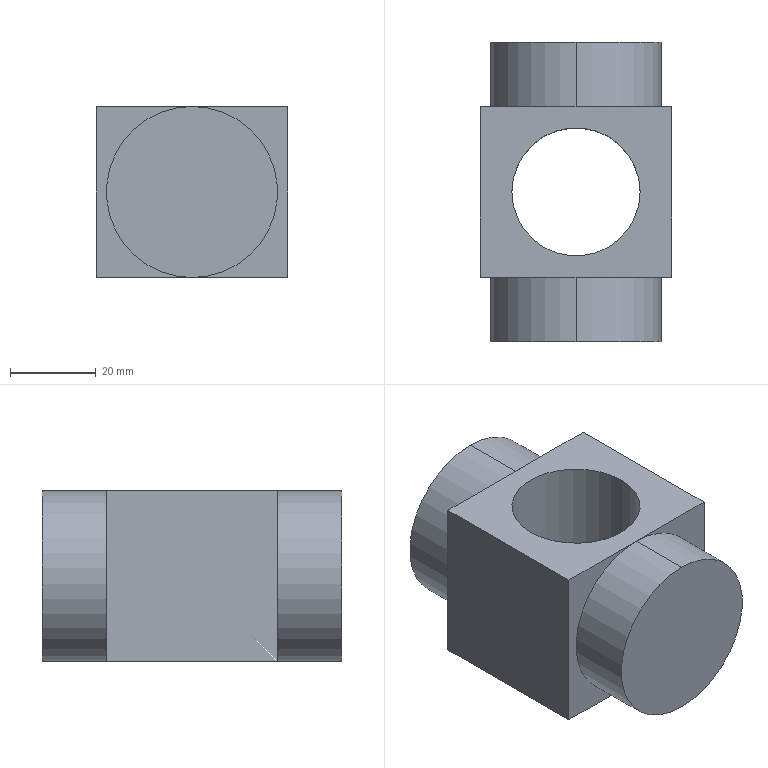Part | SolidWorks | 1 solid | 16 faces | box 44.721 x 70 x 40 mm | volume 80979 mm3 | plane 10 | cylinder 6 | commonest cylinder face diameters 40 x4 30 x2
STEP:
#1=CARTESIAN_POINT('',(-15.,35.,-20.));
#2=VERTEX_POINT('',#1);
#3=CARTESIAN_POINT('',(15.,35.,-20.));
#4=VERTEX_POINT('',#3);
#5=CARTESIAN_POINT('',(0.,35.,-20.));
#6=DIRECTION('',(0.,0.,1.));
#7=DIRECTION('',(-1.,0.,0.));
#8=AXIS2_PLACEMENT_3D('',#5,#6,#7);
#9=CIRCLE('',#8,15.);
#10=EDGE_CURVE('',#2,#4,#9,.T.);
#11=ORIENTED_EDGE('',*,*,#10,.F.);
#12=CARTESIAN_POINT('',(-15.,35.,20.));
#13=VERTEX_POINT('',#12);
#14=CARTESIAN_POINT('',(-15.,35.,-46.5));
#15=DIRECTION('',(0.,0.,1.));
#16=VECTOR('',#15,1000.);
#17=LINE('',#14,#16);
#18=EDGE_CURVE('',#2,#13,#17,.T.);
#19=ORIENTED_EDGE('',*,*,#18,.T.);
#20=CARTESIAN_POINT('',(15.,35.,20.));
#21=VERTEX_POINT('',#20);
#22=CARTESIAN_POINT('',(0.,35.,20.));
#23=DIRECTION('',(0.,0.,-1.));
#24=DIRECTION('',(1.,0.,0.));
#25=AXIS2_PLACEMENT_3D('',#22,#23,#24);
#26=CIRCLE('',#25,15.);
#27=EDGE_CURVE('',#21,#13,#26,.T.);
#28=ORIENTED_EDGE('',*,*,#27,.F.);
#29=CARTESIAN_POINT('',(15.,35.,-46.5));
#30=DIRECTION('',(0.,0.,1.));
#31=VECTOR('',#30,1000.);
#32=LINE('',#29,#31);
#33=EDGE_CURVE('',#4,#21,#32,.T.);
#34=ORIENTED_EDGE('',*,*,#33,.F.);
#35=EDGE_LOOP('',(#11,#19,#28,#34));
#36=FACE_OUTER_BOUND('',#35,.T.);
#37=CARTESIAN_POINT('',(0.,35.,-46.5));
#38=DIRECTION('',(0.,0.,1.));
#39=DIRECTION('',(1.,0.,0.));
#40=AXIS2_PLACEMENT_3D('',#37,#38,#39);
#41=CYLINDRICAL_SURFACE('',#40,15.);
#42=ADVANCED_FACE('',(#36),#41,.F.);
#43=CARTESIAN_POINT('',(0.,15.,-20.));
#44=VERTEX_POINT('',#43);
#45=CARTESIAN_POINT('',(0.,15.,20.));
#46=VERTEX_POINT('',#45);
#47=CARTESIAN_POINT('',(0.,15.,0.));
#48=DIRECTION('',(0.,-1.,0.));
#49=DIRECTION('',(0.,0.,-1.));
#50=AXIS2_PLACEMENT_3D('',#47,#48,#49);
#51=CIRCLE('',#50,20.);
#52=EDGE_CURVE('',#44,#46,#51,.T.);
#53=ORIENTED_EDGE('',*,*,#52,.T.);
#54=CARTESIAN_POINT('',(0.,0.,20.));
#55=VERTEX_POINT('',#54);
#56=CARTESIAN_POINT('',(0.,0.,20.));
#57=DIRECTION('',(0.,-1.,0.));
#58=VECTOR('',#57,1000.);
#59=LINE('',#56,#58);
#60=EDGE_CURVE('',#46,#55,#59,.T.);
#61=ORIENTED_EDGE('',*,*,#60,.T.);
#62=CARTESIAN_POINT('',(0.,0.,-20.));
#63=VERTEX_POINT('',#62);
#64=CARTESIAN_POINT('',(0.,0.,0.));
#65=DIRECTION('',(0.,-1.,0.));
#66=DIRECTION('',(0.,0.,-1.));
#67=AXIS2_PLACEMENT_3D('',#64,#65,#66);
#68=CIRCLE('',#67,20.);
#69=EDGE_CURVE('',#63,#55,#68,.T.);
#70=ORIENTED_EDGE('',*,*,#69,.F.);
#71=CARTESIAN_POINT('',(0.,0.,-20.));
#72=DIRECTION('',(0.,-1.,0.));
#73=VECTOR('',#72,1000.);
#74=LINE('',#71,#73);
#75=EDGE_CURVE('',#44,#63,#74,.T.);
#76=ORIENTED_EDGE('',*,*,#75,.F.);
#77=EDGE_LOOP('',(#53,#61,#70,#76));
#78=FACE_OUTER_BOUND('',#77,.T.);
#79=CARTESIAN_POINT('',(0.,0.,0.));
#80=DIRECTION('',(0.,-1.,0.));
#81=DIRECTION('',(0.,0.,-1.));
#82=AXIS2_PLACEMENT_3D('',#79,#80,#81);
#83=CYLINDRICAL_SURFACE('',#82,20.);
#84=ADVANCED_FACE('',(#78),#83,.T.);
#85=CARTESIAN_POINT('',(0.,70.,-20.));
#86=VERTEX_POINT('',#85);
#87=CARTESIAN_POINT('',(0.,70.,20.));
#88=VERTEX_POINT('',#87);
#89=CARTESIAN_POINT('',(0.,70.,0.));
#90=DIRECTION('',(0.,-1.,0.));
#91=DIRECTION('',(0.,0.,-1.));
#92=AXIS2_PLACEMENT_3D('',#89,#90,#91);
#93=CIRCLE('',#92,20.);
#94=EDGE_CURVE('',#86,#88,#93,.T.);
#95=ORIENTED_EDGE('',*,*,#94,.T.);
#96=CARTESIAN_POINT('',(0.,55.,20.));
#97=VERTEX_POINT('',#96);
#98=CARTESIAN_POINT('',(0.,0.,20.));
#99=DIRECTION('',(0.,-1.,0.));
#100=VECTOR('',#99,1000.);
#101=LINE('',#98,#100);
#102=EDGE_CURVE('',#88,#97,#101,.T.);
#103=ORIENTED_EDGE('',*,*,#102,.T.);
#104=CARTESIAN_POINT('',(0.,55.,-20.));
#105=VERTEX_POINT('',#104);
#106=CARTESIAN_POINT('',(0.,55.,0.));
#107=DIRECTION('',(0.,-1.,0.));
#108=DIRECTION('',(0.,0.,-1.));
#109=AXIS2_PLACEMENT_3D('',#106,#107,#108);
#110=CIRCLE('',#109,20.);
#111=EDGE_CURVE('',#105,#97,#110,.T.);
#112=ORIENTED_EDGE('',*,*,#111,.F.);
#113=CARTESIAN_POINT('',(0.,0.,-20.));
#114=DIRECTION('',(0.,-1.,0.));
#115=VECTOR('',#114,1000.);
#116=LINE('',#113,#115);
#117=EDGE_CURVE('',#86,#105,#116,.T.);
#118=ORIENTED_EDGE('',*,*,#117,.F.);
#119=EDGE_LOOP('',(#95,#103,#112,#118));
#120=FACE_OUTER_BOUND('',#119,.T.);
#121=CARTESIAN_POINT('',(0.,0.,0.));
#122=DIRECTION('',(0.,-1.,0.));
#123=DIRECTION('',(0.,0.,-1.));
#124=AXIS2_PLACEMENT_3D('',#121,#122,#123);
#125=CYLINDRICAL_SURFACE('',#124,20.);
#126=ADVANCED_FACE('',(#120),#125,.T.);
#127=CARTESIAN_POINT('',(22.361,55.,20.));
#128=VERTEX_POINT('',#127);
#129=CARTESIAN_POINT('',(20.,55.,20.));
#130=DIRECTION('',(1.,0.,0.));
#131=VECTOR('',#130,1000.);
#132=LINE('',#129,#131);
#133=EDGE_CURVE('',#97,#128,#132,.T.);
#134=ORIENTED_EDGE('',*,*,#133,.T.);
#135=CARTESIAN_POINT('',(22.361,55.,-20.));
#136=VERTEX_POINT('',#135);
#137=CARTESIAN_POINT('',(22.361,55.,0.));
#138=DIRECTION('',(0.,0.,-1.));
#139=VECTOR('',#138,1000.);
#140=LINE('',#137,#139);
#141=EDGE_CURVE('',#128,#136,#140,.T.);
#142=ORIENTED_EDGE('',*,*,#141,.T.);
#143=CARTESIAN_POINT('',(20.,55.,-20.));
#144=DIRECTION('',(-1.,0.,0.));
#145=VECTOR('',#144,1000.);
#146=LINE('',#143,#145);
#147=EDGE_CURVE('',#136,#105,#146,.T.);
#148=ORIENTED_EDGE('',*,*,#147,.T.);
#149=ORIENTED_EDGE('',*,*,#111,.T.);
#150=EDGE_LOOP('',(#134,#142,#148,#149));
#151=FACE_OUTER_BOUND('',#150,.T.);
#152=CARTESIAN_POINT('',(20.,55.,0.));
#153=DIRECTION('',(0.,1.,0.));
#154=DIRECTION('',(0.,0.,1.));
#155=AXIS2_PLACEMENT_3D('',#152,#153,#154);
#156=PLANE('',#155);
#157=ADVANCED_FACE('',(#151),#156,.T.);
#158=CARTESIAN_POINT('',(0.,55.,0.));
#159=DIRECTION('',(0.,-1.,0.));
#160=DIRECTION('',(0.,0.,-1.));
#161=AXIS2_PLACEMENT_3D('',#158,#159,#160);
#162=CIRCLE('',#161,20.);
#163=EDGE_CURVE('',#97,#105,#162,.T.);
#164=ORIENTED_EDGE('',*,*,#163,.T.);
#165=CARTESIAN_POINT('',(-22.361,55.,-20.));
#166=VERTEX_POINT('',#165);
#167=CARTESIAN_POINT('',(20.,55.,-20.));
#168=DIRECTION('',(-1.,0.,0.));
#169=VECTOR('',#168,1000.);
#170=LINE('',#167,#169);
#171=EDGE_CURVE('',#105,#166,#170,.T.);
#172=ORIENTED_EDGE('',*,*,#171,.T.);
#173=CARTESIAN_POINT('',(-22.361,55.,20.));
#174=VERTEX_POINT('',#173);
#175=CARTESIAN_POINT('',(-22.361,55.,0.));
#176=DIRECTION('',(0.,0.,1.));
#177=VECTOR('',#176,1000.);
#178=LINE('',#175,#177);
#179=EDGE_CURVE('',#166,#174,#178,.T.);
#180=ORIENTED_EDGE('',*,*,#179,.T.);
#181=CARTESIAN_POINT('',(20.,55.,20.));
#182=DIRECTION('',(1.,0.,0.));
#183=VECTOR('',#182,1000.);
#184=LINE('',#181,#183);
#185=EDGE_CURVE('',#174,#97,#184,.T.);
#186=ORIENTED_EDGE('',*,*,#185,.T.);
#187=EDGE_LOOP('',(#164,#172,#180,#186));
#188=FACE_OUTER_BOUND('',#187,.T.);
#189=CARTESIAN_POINT('',(20.,55.,0.));
#190=DIRECTION('',(0.,1.,0.));
#191=DIRECTION('',(0.,0.,1.));
#192=AXIS2_PLACEMENT_3D('',#189,#190,#191);
#193=PLANE('',#192);
#194=ADVANCED_FACE('',(#188),#193,.T.);
#195=ORIENTED_EDGE('',*,*,#94,.F.);
#196=CARTESIAN_POINT('',(0.,70.,0.));
#197=DIRECTION('',(0.,-1.,0.));
#198=DIRECTION('',(0.,0.,-1.));
#199=AXIS2_PLACEMENT_3D('',#196,#197,#198);
#200=CIRCLE('',#199,20.);
#201=EDGE_CURVE('',#88,#86,#200,.T.);
#202=ORIENTED_EDGE('',*,*,#201,.F.);
#203=EDGE_LOOP('',(#195,#202));
#204=FACE_OUTER_BOUND('',#203,.T.);
#205=CARTESIAN_POINT('',(0.,70.,0.));
#206=DIRECTION('',(0.,1.,0.));
#207=DIRECTION('',(0.,0.,1.));
#208=AXIS2_PLACEMENT_3D('',#205,#206,#207);
#209=PLANE('',#208);
#210=ADVANCED_FACE('',(#204),#209,.T.);
#211=ORIENTED_EDGE('',*,*,#102,.F.);
#212=ORIENTED_EDGE('',*,*,#201,.T.);
#213=ORIENTED_EDGE('',*,*,#117,.T.);
#214=ORIENTED_EDGE('',*,*,#163,.F.);
#215=EDGE_LOOP('',(#211,#212,#213,#214));
#216=FACE_OUTER_BOUND('',#215,.T.);
#217=CARTESIAN_POINT('',(0.,0.,0.));
#218=DIRECTION('',(0.,-1.,0.));
#219=DIRECTION('',(0.,0.,-1.));
#220=AXIS2_PLACEMENT_3D('',#217,#218,#219);
#221=CYLINDRICAL_SURFACE('',#220,20.);
#222=ADVANCED_FACE('',(#216),#221,.T.);
#223=CARTESIAN_POINT('',(22.361,15.,-20.));
#224=VERTEX_POINT('',#223);
#225=CARTESIAN_POINT('',(22.361,61.5,-20.));
#226=DIRECTION('',(0.,-1.,0.));
#227=VECTOR('',#226,1000.);
#228=LINE('',#225,#227);
#229=EDGE_CURVE('',#136,#224,#228,.T.);
#230=ORIENTED_EDGE('',*,*,#229,.T.);
#231=CARTESIAN_POINT('',(30.,15.,-20.));
#232=DIRECTION('',(1.,0.,0.));
#233=VECTOR('',#232,1000.);
#234=LINE('',#231,#233);
#235=EDGE_CURVE('',#44,#224,#234,.T.);
#236=ORIENTED_EDGE('',*,*,#235,.F.);
#237=CARTESIAN_POINT('',(-22.361,15.,-20.));
#238=VERTEX_POINT('',#237);
#239=CARTESIAN_POINT('',(30.,15.,-20.));
#240=DIRECTION('',(1.,0.,0.));
#241=VECTOR('',#240,1000.);
#242=LINE('',#239,#241);
#243=EDGE_CURVE('',#238,#44,#242,.T.);
#244=ORIENTED_EDGE('',*,*,#243,.F.);
#245=CARTESIAN_POINT('',(-22.361,61.5,-20.));
#246=DIRECTION('',(0.,-1.,0.));
#247=VECTOR('',#246,1000.);
#248=LINE('',#245,#247);
#249=EDGE_CURVE('',#166,#238,#248,.T.);
#250=ORIENTED_EDGE('',*,*,#249,.F.);
#251=ORIENTED_EDGE('',*,*,#171,.F.);
#252=ORIENTED_EDGE('',*,*,#147,.F.);
#253=EDGE_LOOP('',(#230,#236,#244,#250,#251,#252));
#254=FACE_OUTER_BOUND('',#253,.T.);
#255=CARTESIAN_POINT('',(0.,35.,-20.));
#256=DIRECTION('',(0.,0.,1.));
#257=DIRECTION('',(-1.,0.,0.));
#258=AXIS2_PLACEMENT_3D('',#255,#256,#257);
#259=CIRCLE('',#258,15.);
#260=EDGE_CURVE('',#4,#2,#259,.T.);
#261=ORIENTED_EDGE('',*,*,#260,.T.);
#262=ORIENTED_EDGE('',*,*,#10,.T.);
#263=EDGE_LOOP('',(#261,#262));
#264=FACE_BOUND('',#263,.T.);
#265=CARTESIAN_POINT('',(-22.361,61.5,-20.));
#266=DIRECTION('',(0.,0.,-1.));
#267=DIRECTION('',(-1.,0.,0.));
#268=AXIS2_PLACEMENT_3D('',#265,#266,#267);
#269=PLANE('',#268);
#270=ADVANCED_FACE('',(#254,#264),#269,.T.);
#271=CARTESIAN_POINT('',(-22.361,15.,20.));
#272=VERTEX_POINT('',#271);
#273=CARTESIAN_POINT('',(-22.361,61.5,20.));
#274=DIRECTION('',(0.,-1.,0.));
#275=VECTOR('',#274,1000.);
#276=LINE('',#273,#275);
#277=EDGE_CURVE('',#174,#272,#276,.T.);
#278=ORIENTED_EDGE('',*,*,#277,.T.);
#279=CARTESIAN_POINT('',(30.,15.,20.));
#280=DIRECTION('',(-1.,0.,0.));
#281=VECTOR('',#280,1000.);
#282=LINE('',#279,#281);
#283=EDGE_CURVE('',#46,#272,#282,.T.);
#284=ORIENTED_EDGE('',*,*,#283,.F.);
#285=CARTESIAN_POINT('',(22.361,15.,20.));
#286=VERTEX_POINT('',#285);
#287=CARTESIAN_POINT('',(30.,15.,20.));
#288=DIRECTION('',(-1.,0.,0.));
#289=VECTOR('',#288,1000.);
#290=LINE('',#287,#289);
#291=EDGE_CURVE('',#286,#46,#290,.T.);
#292=ORIENTED_EDGE('',*,*,#291,.F.);
#293=CARTESIAN_POINT('',(22.361,61.5,20.));
#294=DIRECTION('',(0.,-1.,0.));
#295=VECTOR('',#294,1000.);
#296=LINE('',#293,#295);
#297=EDGE_CURVE('',#128,#286,#296,.T.);
#298=ORIENTED_EDGE('',*,*,#297,.F.);
#299=ORIENTED_EDGE('',*,*,#133,.F.);
#300=ORIENTED_EDGE('',*,*,#185,.F.);
#301=EDGE_LOOP('',(#278,#284,#292,#298,#299,#300));
#302=FACE_OUTER_BOUND('',#301,.T.);
#303=ORIENTED_EDGE('',*,*,#27,.T.);
#304=CARTESIAN_POINT('',(0.,35.,20.));
#305=DIRECTION('',(0.,0.,-1.));
#306=DIRECTION('',(1.,0.,0.));
#307=AXIS2_PLACEMENT_3D('',#304,#305,#306);
#308=CIRCLE('',#307,15.);
#309=EDGE_CURVE('',#13,#21,#308,.T.);
#310=ORIENTED_EDGE('',*,*,#309,.T.);
#311=EDGE_LOOP('',(#303,#310));
#312=FACE_BOUND('',#311,.T.);
#313=CARTESIAN_POINT('',(-22.361,61.5,20.));
#314=DIRECTION('',(0.,0.,1.));
#315=DIRECTION('',(1.,0.,0.));
#316=AXIS2_PLACEMENT_3D('',#313,#314,#315);
#317=PLANE('',#316);
#318=ADVANCED_FACE('',(#302,#312),#317,.T.);
#319=ORIENTED_EDGE('',*,*,#297,.T.);
#320=CARTESIAN_POINT('',(22.361,15.,0.));
#321=DIRECTION('',(0.,0.,1.));
#322=VECTOR('',#321,1000.);
#323=LINE('',#320,#322);
#324=EDGE_CURVE('',#224,#286,#323,.T.);
#325=ORIENTED_EDGE('',*,*,#324,.F.);
#326=ORIENTED_EDGE('',*,*,#229,.F.);
#327=ORIENTED_EDGE('',*,*,#141,.F.);
#328=EDGE_LOOP('',(#319,#325,#326,#327));
#329=FACE_OUTER_BOUND('',#328,.T.);
#330=CARTESIAN_POINT('',(22.361,61.5,20.));
#331=DIRECTION('',(1.,0.,0.));
#332=DIRECTION('',(0.,0.,-1.));
#333=AXIS2_PLACEMENT_3D('',#330,#331,#332);
#334=PLANE('',#333);
#335=ADVANCED_FACE('',(#329),#334,.T.);
#336=ORIENTED_EDGE('',*,*,#249,.T.);
#337=CARTESIAN_POINT('',(-22.361,15.,0.));
#338=DIRECTION('',(0.,0.,-1.));
#339=VECTOR('',#338,1000.);
#340=LINE('',#337,#339);
#341=EDGE_CURVE('',#272,#238,#340,.T.);
#342=ORIENTED_EDGE('',*,*,#341,.F.);
#343=ORIENTED_EDGE('',*,*,#277,.F.);
#344=ORIENTED_EDGE('',*,*,#179,.F.);
#345=EDGE_LOOP('',(#336,#342,#343,#344));
#346=FACE_OUTER_BOUND('',#345,.T.);
#347=CARTESIAN_POINT('',(-22.361,61.5,20.));
#348=DIRECTION('',(-1.,0.,0.));
#349=DIRECTION('',(0.,0.,1.));
#350=AXIS2_PLACEMENT_3D('',#347,#348,#349);
#351=PLANE('',#350);
#352=ADVANCED_FACE('',(#346),#351,.T.);
#353=ORIENTED_EDGE('',*,*,#69,.T.);
#354=CARTESIAN_POINT('',(0.,0.,0.));
#355=DIRECTION('',(0.,-1.,0.));
#356=DIRECTION('',(0.,0.,-1.));
#357=AXIS2_PLACEMENT_3D('',#354,#355,#356);
#358=CIRCLE('',#357,20.);
#359=EDGE_CURVE('',#55,#63,#358,.T.);
#360=ORIENTED_EDGE('',*,*,#359,.T.);
#361=EDGE_LOOP('',(#353,#360));
#362=FACE_OUTER_BOUND('',#361,.T.);
#363=CARTESIAN_POINT('',(20.,0.,0.));
#364=DIRECTION('',(0.,-1.,0.));
#365=DIRECTION('',(0.,0.,-1.));
#366=AXIS2_PLACEMENT_3D('',#363,#364,#365);
#367=PLANE('',#366);
#368=ADVANCED_FACE('',(#362),#367,.T.);
#369=ORIENTED_EDGE('',*,*,#60,.F.);
#370=CARTESIAN_POINT('',(0.,15.,0.));
#371=DIRECTION('',(0.,-1.,0.));
#372=DIRECTION('',(0.,0.,-1.));
#373=AXIS2_PLACEMENT_3D('',#370,#371,#372);
#374=CIRCLE('',#373,20.);
#375=EDGE_CURVE('',#46,#44,#374,.T.);
#376=ORIENTED_EDGE('',*,*,#375,.T.);
#377=ORIENTED_EDGE('',*,*,#75,.T.);
#378=ORIENTED_EDGE('',*,*,#359,.F.);
#379=EDGE_LOOP('',(#369,#376,#377,#378));
#380=FACE_OUTER_BOUND('',#379,.T.);
#381=CARTESIAN_POINT('',(0.,0.,0.));
#382=DIRECTION('',(0.,-1.,0.));
#383=DIRECTION('',(0.,0.,-1.));
#384=AXIS2_PLACEMENT_3D('',#381,#382,#383);
#385=CYLINDRICAL_SURFACE('',#384,20.);
#386=ADVANCED_FACE('',(#380),#385,.T.);
#387=ORIENTED_EDGE('',*,*,#341,.T.);
#388=ORIENTED_EDGE('',*,*,#243,.T.);
#389=ORIENTED_EDGE('',*,*,#375,.F.);
#390=ORIENTED_EDGE('',*,*,#283,.T.);
#391=EDGE_LOOP('',(#387,#388,#389,#390));
#392=FACE_OUTER_BOUND('',#391,.T.);
#393=CARTESIAN_POINT('',(30.,15.,0.));
#394=DIRECTION('',(0.,-1.,0.));
#395=DIRECTION('',(0.,0.,-1.));
#396=AXIS2_PLACEMENT_3D('',#393,#394,#395);
#397=PLANE('',#396);
#398=ADVANCED_FACE('',(#392),#397,.T.);
#399=ORIENTED_EDGE('',*,*,#52,.F.);
#400=ORIENTED_EDGE('',*,*,#235,.T.);
#401=ORIENTED_EDGE('',*,*,#324,.T.);
#402=ORIENTED_EDGE('',*,*,#291,.T.);
#403=EDGE_LOOP('',(#399,#400,#401,#402));
#404=FACE_OUTER_BOUND('',#403,.T.);
#405=CARTESIAN_POINT('',(30.,15.,0.));
#406=DIRECTION('',(0.,-1.,0.));
#407=DIRECTION('',(0.,0.,-1.));
#408=AXIS2_PLACEMENT_3D('',#405,#406,#407);
#409=PLANE('',#408);
#410=ADVANCED_FACE('',(#404),#409,.T.);
#411=ORIENTED_EDGE('',*,*,#18,.F.);
#412=ORIENTED_EDGE('',*,*,#260,.F.);
#413=ORIENTED_EDGE('',*,*,#33,.T.);
#414=ORIENTED_EDGE('',*,*,#309,.F.);
#415=EDGE_LOOP('',(#411,#412,#413,#414));
#416=FACE_OUTER_BOUND('',#415,.T.);
#417=CARTESIAN_POINT('',(0.,35.,-46.5));
#418=DIRECTION('',(0.,0.,1.));
#419=DIRECTION('',(1.,0.,0.));
#420=AXIS2_PLACEMENT_3D('',#417,#418,#419);
#421=CYLINDRICAL_SURFACE('',#420,15.);
#422=ADVANCED_FACE('',(#416),#421,.F.);
#423=CLOSED_SHELL('',(#42,#84,#126,#157,#194,#210,#222,#270,#318,#335,#352,#368,#386,#398,#410,#422));
#424=MANIFOLD_SOLID_BREP('',#423);
#425=CARTESIAN_POINT('',(0.,0.,0.));
#426=DIRECTION('',(0.,0.,1.));
#427=DIRECTION('',(1.,0.,0.));
#428=AXIS2_PLACEMENT_3D('',#425,#426,#427);
#429=(LENGTH_UNIT()NAMED_UNIT(*)SI_UNIT(.MILLI.,.METRE.));
#430=UNCERTAINTY_MEASURE_WITH_UNIT(LENGTH_MEASURE(0.00001),#429,'','');
#431=(NAMED_UNIT(*)PLANE_ANGLE_UNIT()SI_UNIT($,.RADIAN.));
#432=(NAMED_UNIT(*)SI_UNIT($,.STERADIAN.)SOLID_ANGLE_UNIT());
#433=(GEOMETRIC_REPRESENTATION_CONTEXT(3)GLOBAL_UNCERTAINTY_ASSIGNED_CONTEXT((#430))GLOBAL_UNIT_ASSIGNED_CONTEXT((#429,#431,#432))REPRESENTATION_CONTEXT('',''));
#434=ADVANCED_BREP_SHAPE_REPRESENTATION('',(#424,#428),#433);